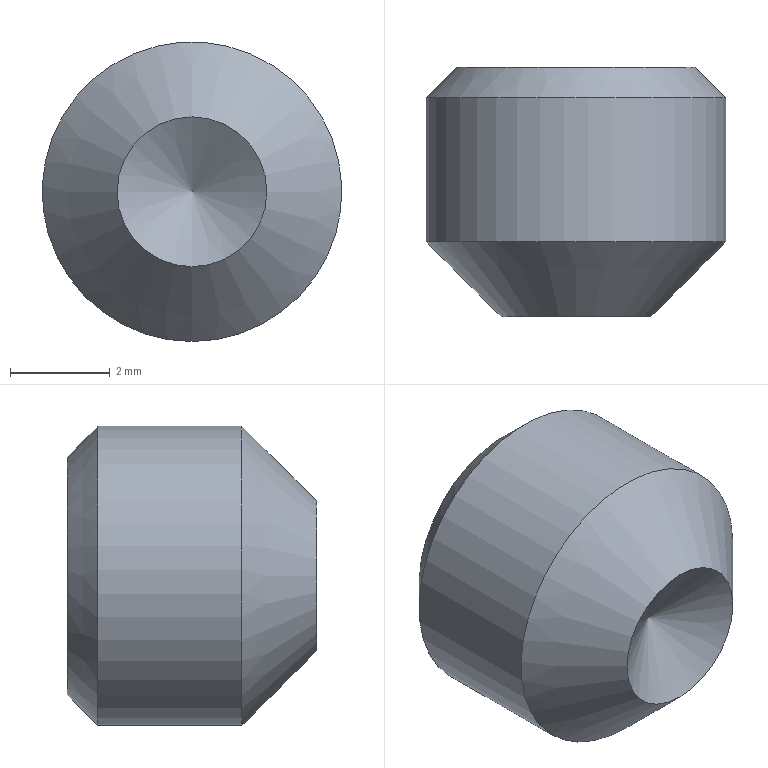Part | NX | features 5003_344_MSSU6-5(Default) 2 | 1 solid | 12 faces | box 6 x 5 x 6 mm | volume 102.686 mm3 | plane 8 | cone 3 | cylinder 1 | commonest cylinder face diameters 6 x1
STEP:
#1=CARTESIAN_POINT('',(-1.341,141.5,-148.5));
#2=VERTEX_POINT('',#1);
#3=CARTESIAN_POINT('',(-2.207,141.5,-147.));
#4=VERTEX_POINT('',#3);
#5=CARTESIAN_POINT('',(-1.341,141.5,-148.5));
#6=DIRECTION('',(-0.5,0.,0.866));
#7=VECTOR('',#6,1000.);
#8=LINE('',#5,#7);
#9=EDGE_CURVE('',#2,#4,#8,.T.);
#10=ORIENTED_EDGE('',*,*,#9,.F.);
#11=CARTESIAN_POINT('',(0.391,141.5,-148.5));
#12=VERTEX_POINT('',#11);
#13=CARTESIAN_POINT('',(0.391,141.5,-148.5));
#14=DIRECTION('',(-1.,0.,0.));
#15=VECTOR('',#14,1000.);
#16=LINE('',#13,#15);
#17=EDGE_CURVE('',#12,#2,#16,.T.);
#18=ORIENTED_EDGE('',*,*,#17,.F.);
#19=CARTESIAN_POINT('',(1.257,141.5,-147.));
#20=VERTEX_POINT('',#19);
#21=CARTESIAN_POINT('',(1.257,141.5,-147.));
#22=DIRECTION('',(-0.5,0.,-0.866));
#23=VECTOR('',#22,1000.);
#24=LINE('',#21,#23);
#25=EDGE_CURVE('',#20,#12,#24,.T.);
#26=ORIENTED_EDGE('',*,*,#25,.F.);
#27=CARTESIAN_POINT('',(0.391,141.5,-145.5));
#28=VERTEX_POINT('',#27);
#29=CARTESIAN_POINT('',(0.391,141.5,-145.5));
#30=DIRECTION('',(0.5,0.,-0.866));
#31=VECTOR('',#30,1000.);
#32=LINE('',#29,#31);
#33=EDGE_CURVE('',#28,#20,#32,.T.);
#34=ORIENTED_EDGE('',*,*,#33,.F.);
#35=CARTESIAN_POINT('',(-1.341,141.5,-145.5));
#36=VERTEX_POINT('',#35);
#37=CARTESIAN_POINT('',(-1.341,141.5,-145.5));
#38=DIRECTION('',(1.,0.,0.));
#39=VECTOR('',#38,1000.);
#40=LINE('',#37,#39);
#41=EDGE_CURVE('',#36,#28,#40,.T.);
#42=ORIENTED_EDGE('',*,*,#41,.F.);
#43=CARTESIAN_POINT('',(-2.207,141.5,-147.));
#44=DIRECTION('',(0.5,0.,0.866));
#45=VECTOR('',#44,1000.);
#46=LINE('',#43,#45);
#47=EDGE_CURVE('',#4,#36,#46,.T.);
#48=ORIENTED_EDGE('',*,*,#47,.F.);
#49=EDGE_LOOP('',(#10,#18,#26,#34,#42,#48));
#50=FACE_BOUND('',#49,.T.);
#51=CARTESIAN_POINT('',(-0.475,141.5,-149.387));
#52=VERTEX_POINT('',#51);
#53=CARTESIAN_POINT('',(-0.475,141.5,-147.));
#54=DIRECTION('',(0.,1.,0.));
#55=DIRECTION('',(0.,0.,-1.));
#56=AXIS2_PLACEMENT_3D('',#53,#54,#55);
#57=CIRCLE('',#56,2.386);
#58=EDGE_CURVE('',#52,#52,#57,.T.);
#59=ORIENTED_EDGE('',*,*,#58,.T.);
#60=EDGE_LOOP('',(#59));
#61=FACE_BOUND('',#60,.T.);
#62=CARTESIAN_POINT('',(1.912,141.5,-147.));
#63=DIRECTION('',(0.,1.,0.));
#64=DIRECTION('',(0.,0.,-1.));
#65=AXIS2_PLACEMENT_3D('',#62,#63,#64);
#66=PLANE('',#65);
#67=ADVANCED_FACE('',(#50,#61),#66,.T.);
#68=CARTESIAN_POINT('',(-1.975,136.5,-147.));
#69=VERTEX_POINT('',#68);
#70=CARTESIAN_POINT('',(-0.475,136.5,-147.));
#71=DIRECTION('',(0.,-1.,0.));
#72=DIRECTION('',(-1.,0.,0.));
#73=AXIS2_PLACEMENT_3D('',#70,#71,#72);
#74=CIRCLE('',#73,1.5);
#75=EDGE_CURVE('',#69,#69,#74,.T.);
#76=ORIENTED_EDGE('',*,*,#75,.F.);
#77=EDGE_LOOP('',(#76));
#78=FACE_BOUND('',#77,.T.);
#79=CARTESIAN_POINT('',(-0.475,138.,-150.));
#80=VERTEX_POINT('',#79);
#81=CARTESIAN_POINT('',(-0.475,138.,-147.));
#82=DIRECTION('',(0.,1.,0.));
#83=DIRECTION('',(0.,0.,-1.));
#84=AXIS2_PLACEMENT_3D('',#81,#82,#83);
#85=CIRCLE('',#84,3.);
#86=EDGE_CURVE('',#80,#80,#85,.T.);
#87=ORIENTED_EDGE('',*,*,#86,.F.);
#88=EDGE_LOOP('',(#87));
#89=FACE_BOUND('',#88,.T.);
#90=CARTESIAN_POINT('',(-0.475,138.,-147.));
#91=DIRECTION('',(0.,1.,0.));
#92=DIRECTION('',(0.,0.,-1.));
#93=AXIS2_PLACEMENT_3D('',#90,#91,#92);
#94=CONICAL_SURFACE('',#93,3.,0.7854);
#95=ADVANCED_FACE('',(#78,#89),#94,.T.);
#96=ORIENTED_EDGE('',*,*,#86,.T.);
#97=EDGE_LOOP('',(#96));
#98=FACE_BOUND('',#97,.T.);
#99=CARTESIAN_POINT('',(-0.475,140.887,-150.));
#100=VERTEX_POINT('',#99);
#101=CARTESIAN_POINT('',(-0.475,140.887,-147.));
#102=DIRECTION('',(0.,1.,0.));
#103=DIRECTION('',(0.,0.,-1.));
#104=AXIS2_PLACEMENT_3D('',#101,#102,#103);
#105=CIRCLE('',#104,3.);
#106=EDGE_CURVE('',#100,#100,#105,.T.);
#107=ORIENTED_EDGE('',*,*,#106,.F.);
#108=EDGE_LOOP('',(#107));
#109=FACE_BOUND('',#108,.T.);
#110=CARTESIAN_POINT('',(-0.475,141.75,-147.));
#111=DIRECTION('',(0.,1.,0.));
#112=DIRECTION('',(0.,0.,-1.));
#113=AXIS2_PLACEMENT_3D('',#110,#111,#112);
#114=CYLINDRICAL_SURFACE('',#113,3.);
#115=ADVANCED_FACE('',(#98,#109),#114,.T.);
#116=ORIENTED_EDGE('',*,*,#106,.T.);
#117=EDGE_LOOP('',(#116));
#118=FACE_BOUND('',#117,.T.);
#119=ORIENTED_EDGE('',*,*,#58,.F.);
#120=EDGE_LOOP('',(#119));
#121=FACE_BOUND('',#120,.T.);
#122=CARTESIAN_POINT('',(-0.475,141.5,-147.));
#123=DIRECTION('',(0.,-1.,0.));
#124=DIRECTION('',(0.,0.,1.));
#125=AXIS2_PLACEMENT_3D('',#122,#123,#124);
#126=CONICAL_SURFACE('',#125,2.386,0.7854);
#127=ADVANCED_FACE('',(#118,#121),#126,.T.);
#128=ORIENTED_EDGE('',*,*,#9,.T.);
#129=CARTESIAN_POINT('',(-2.207,139.5,-147.));
#130=VERTEX_POINT('',#129);
#131=CARTESIAN_POINT('',(-2.207,139.5,-147.));
#132=DIRECTION('',(0.,1.,0.));
#133=VECTOR('',#132,1000.);
#134=LINE('',#131,#133);
#135=EDGE_CURVE('',#130,#4,#134,.T.);
#136=ORIENTED_EDGE('',*,*,#135,.F.);
#137=CARTESIAN_POINT('',(-1.341,139.5,-148.5));
#138=VERTEX_POINT('',#137);
#139=CARTESIAN_POINT('',(-1.341,139.5,-148.5));
#140=DIRECTION('',(-0.5,0.,0.866));
#141=VECTOR('',#140,1000.);
#142=LINE('',#139,#141);
#143=EDGE_CURVE('',#138,#130,#142,.T.);
#144=ORIENTED_EDGE('',*,*,#143,.F.);
#145=CARTESIAN_POINT('',(-1.341,139.5,-148.5));
#146=DIRECTION('',(0.,1.,0.));
#147=VECTOR('',#146,1000.);
#148=LINE('',#145,#147);
#149=EDGE_CURVE('',#138,#2,#148,.T.);
#150=ORIENTED_EDGE('',*,*,#149,.T.);
#151=EDGE_LOOP('',(#128,#136,#144,#150));
#152=FACE_BOUND('',#151,.T.);
#153=CARTESIAN_POINT('',(-1.341,139.5,-148.5));
#154=DIRECTION('',(-0.866,0.,-0.5));
#155=DIRECTION('',(0.5,0.,-0.866));
#156=AXIS2_PLACEMENT_3D('',#153,#154,#155);
#157=PLANE('',#156);
#158=ADVANCED_FACE('',(#152),#157,.F.);
#159=ORIENTED_EDGE('',*,*,#17,.T.);
#160=ORIENTED_EDGE('',*,*,#149,.F.);
#161=CARTESIAN_POINT('',(0.391,139.5,-148.5));
#162=VERTEX_POINT('',#161);
#163=CARTESIAN_POINT('',(0.391,139.5,-148.5));
#164=DIRECTION('',(-1.,0.,0.));
#165=VECTOR('',#164,1000.);
#166=LINE('',#163,#165);
#167=EDGE_CURVE('',#162,#138,#166,.T.);
#168=ORIENTED_EDGE('',*,*,#167,.F.);
#169=CARTESIAN_POINT('',(0.391,139.5,-148.5));
#170=DIRECTION('',(0.,1.,0.));
#171=VECTOR('',#170,1000.);
#172=LINE('',#169,#171);
#173=EDGE_CURVE('',#162,#12,#172,.T.);
#174=ORIENTED_EDGE('',*,*,#173,.T.);
#175=EDGE_LOOP('',(#159,#160,#168,#174));
#176=FACE_BOUND('',#175,.T.);
#177=CARTESIAN_POINT('',(0.391,139.5,-148.5));
#178=DIRECTION('',(0.,0.,-1.));
#179=DIRECTION('',(1.,0.,0.));
#180=AXIS2_PLACEMENT_3D('',#177,#178,#179);
#181=PLANE('',#180);
#182=ADVANCED_FACE('',(#176),#181,.F.);
#183=ORIENTED_EDGE('',*,*,#25,.T.);
#184=ORIENTED_EDGE('',*,*,#173,.F.);
#185=CARTESIAN_POINT('',(1.257,139.5,-147.));
#186=VERTEX_POINT('',#185);
#187=CARTESIAN_POINT('',(1.257,139.5,-147.));
#188=DIRECTION('',(-0.5,0.,-0.866));
#189=VECTOR('',#188,1000.);
#190=LINE('',#187,#189);
#191=EDGE_CURVE('',#186,#162,#190,.T.);
#192=ORIENTED_EDGE('',*,*,#191,.F.);
#193=CARTESIAN_POINT('',(1.257,139.5,-147.));
#194=DIRECTION('',(0.,1.,0.));
#195=VECTOR('',#194,1000.);
#196=LINE('',#193,#195);
#197=EDGE_CURVE('',#186,#20,#196,.T.);
#198=ORIENTED_EDGE('',*,*,#197,.T.);
#199=EDGE_LOOP('',(#183,#184,#192,#198));
#200=FACE_BOUND('',#199,.T.);
#201=CARTESIAN_POINT('',(1.257,139.5,-147.));
#202=DIRECTION('',(0.866,0.,-0.5));
#203=DIRECTION('',(0.5,0.,0.866));
#204=AXIS2_PLACEMENT_3D('',#201,#202,#203);
#205=PLANE('',#204);
#206=ADVANCED_FACE('',(#200),#205,.F.);
#207=ORIENTED_EDGE('',*,*,#33,.T.);
#208=ORIENTED_EDGE('',*,*,#197,.F.);
#209=CARTESIAN_POINT('',(0.391,139.5,-145.5));
#210=VERTEX_POINT('',#209);
#211=CARTESIAN_POINT('',(0.391,139.5,-145.5));
#212=DIRECTION('',(0.5,0.,-0.866));
#213=VECTOR('',#212,1000.);
#214=LINE('',#211,#213);
#215=EDGE_CURVE('',#210,#186,#214,.T.);
#216=ORIENTED_EDGE('',*,*,#215,.F.);
#217=CARTESIAN_POINT('',(0.391,139.5,-145.5));
#218=DIRECTION('',(0.,1.,0.));
#219=VECTOR('',#218,1000.);
#220=LINE('',#217,#219);
#221=EDGE_CURVE('',#210,#28,#220,.T.);
#222=ORIENTED_EDGE('',*,*,#221,.T.);
#223=EDGE_LOOP('',(#207,#208,#216,#222));
#224=FACE_BOUND('',#223,.T.);
#225=CARTESIAN_POINT('',(0.391,139.5,-145.5));
#226=DIRECTION('',(0.866,0.,0.5));
#227=DIRECTION('',(-0.5,0.,0.866));
#228=AXIS2_PLACEMENT_3D('',#225,#226,#227);
#229=PLANE('',#228);
#230=ADVANCED_FACE('',(#224),#229,.F.);
#231=ORIENTED_EDGE('',*,*,#41,.T.);
#232=ORIENTED_EDGE('',*,*,#221,.F.);
#233=CARTESIAN_POINT('',(-1.341,139.5,-145.5));
#234=VERTEX_POINT('',#233);
#235=CARTESIAN_POINT('',(-1.341,139.5,-145.5));
#236=DIRECTION('',(1.,0.,0.));
#237=VECTOR('',#236,1000.);
#238=LINE('',#235,#237);
#239=EDGE_CURVE('',#234,#210,#238,.T.);
#240=ORIENTED_EDGE('',*,*,#239,.F.);
#241=CARTESIAN_POINT('',(-1.341,139.5,-145.5));
#242=DIRECTION('',(0.,1.,0.));
#243=VECTOR('',#242,1000.);
#244=LINE('',#241,#243);
#245=EDGE_CURVE('',#234,#36,#244,.T.);
#246=ORIENTED_EDGE('',*,*,#245,.T.);
#247=EDGE_LOOP('',(#231,#232,#240,#246));
#248=FACE_BOUND('',#247,.T.);
#249=CARTESIAN_POINT('',(-1.341,139.5,-145.5));
#250=DIRECTION('',(0.,0.,1.));
#251=DIRECTION('',(0.,1.,0.));
#252=AXIS2_PLACEMENT_3D('',#249,#250,#251);
#253=PLANE('',#252);
#254=ADVANCED_FACE('',(#248),#253,.F.);
#255=ORIENTED_EDGE('',*,*,#47,.T.);
#256=ORIENTED_EDGE('',*,*,#245,.F.);
#257=CARTESIAN_POINT('',(-2.207,139.5,-147.));
#258=DIRECTION('',(0.5,0.,0.866));
#259=VECTOR('',#258,1000.);
#260=LINE('',#257,#259);
#261=EDGE_CURVE('',#130,#234,#260,.T.);
#262=ORIENTED_EDGE('',*,*,#261,.F.);
#263=ORIENTED_EDGE('',*,*,#135,.T.);
#264=EDGE_LOOP('',(#255,#256,#262,#263));
#265=FACE_BOUND('',#264,.T.);
#266=CARTESIAN_POINT('',(-2.207,139.5,-147.));
#267=DIRECTION('',(-0.866,0.,0.5));
#268=DIRECTION('',(-0.5,0.,-0.866));
#269=AXIS2_PLACEMENT_3D('',#266,#267,#268);
#270=PLANE('',#269);
#271=ADVANCED_FACE('',(#265),#270,.F.);
#272=ORIENTED_EDGE('',*,*,#143,.T.);
#273=ORIENTED_EDGE('',*,*,#261,.T.);
#274=ORIENTED_EDGE('',*,*,#239,.T.);
#275=ORIENTED_EDGE('',*,*,#215,.T.);
#276=ORIENTED_EDGE('',*,*,#191,.T.);
#277=ORIENTED_EDGE('',*,*,#167,.T.);
#278=EDGE_LOOP('',(#272,#273,#274,#275,#276,#277));
#279=FACE_BOUND('',#278,.T.);
#280=CARTESIAN_POINT('',(-0.475,139.5,-147.));
#281=DIRECTION('',(0.,1.,0.));
#282=DIRECTION('',(0.,0.,-1.));
#283=AXIS2_PLACEMENT_3D('',#280,#281,#282);
#284=PLANE('',#283);
#285=ADVANCED_FACE('',(#279),#284,.T.);
#286=ORIENTED_EDGE('',*,*,#75,.T.);
#287=EDGE_LOOP('',(#286));
#288=FACE_BOUND('',#287,.T.);
#289=CARTESIAN_POINT('',(-0.475,137.4,-147.));
#290=VERTEX_POINT('',#289);
#291=VERTEX_LOOP('',#290);
#292=FACE_BOUND('',#291,.T.);
#293=CARTESIAN_POINT('',(-0.475,137.4,-147.));
#294=DIRECTION('',(0.,-1.,0.));
#295=DIRECTION('',(-1.,0.,0.));
#296=AXIS2_PLACEMENT_3D('',#293,#294,#295);
#297=CONICAL_SURFACE('',#296,0.,1.03);
#298=ADVANCED_FACE('',(#288,#292),#297,.F.);
#299=CLOSED_SHELL('',(#67,#95,#115,#127,#158,#182,#206,#230,#254,#271,#285,#298));
#300=MANIFOLD_SOLID_BREP('',#299);
#301=(LENGTH_UNIT()NAMED_UNIT(*)SI_UNIT(.MILLI.,.METRE.));
#302=UNCERTAINTY_MEASURE_WITH_UNIT(LENGTH_MEASURE(0.00001),#301,'','');
#303=(NAMED_UNIT(*)PLANE_ANGLE_UNIT()SI_UNIT($,.RADIAN.));
#304=(NAMED_UNIT(*)SI_UNIT($,.STERADIAN.)SOLID_ANGLE_UNIT());
#305=(GEOMETRIC_REPRESENTATION_CONTEXT(3)GLOBAL_UNCERTAINTY_ASSIGNED_CONTEXT((#302))GLOBAL_UNIT_ASSIGNED_CONTEXT((#301,#303,#304))REPRESENTATION_CONTEXT('',''));
#306=ADVANCED_BREP_SHAPE_REPRESENTATION('',(#300),#305);